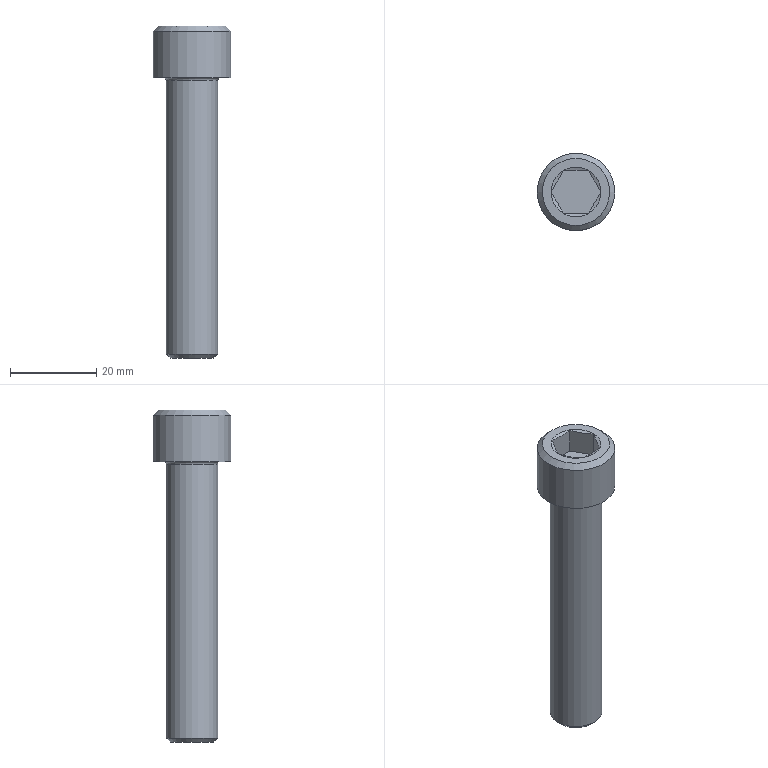Part | STEP file | solid 136 | 1 solid | 21 faces | box 18 x 18 x 77 mm | volume 9833 mm3 | plane 10 | sphere 6 | cylinder 2 | cone 2 | torus 1 | commonest cylinder face diameters 12 x1 18 x1